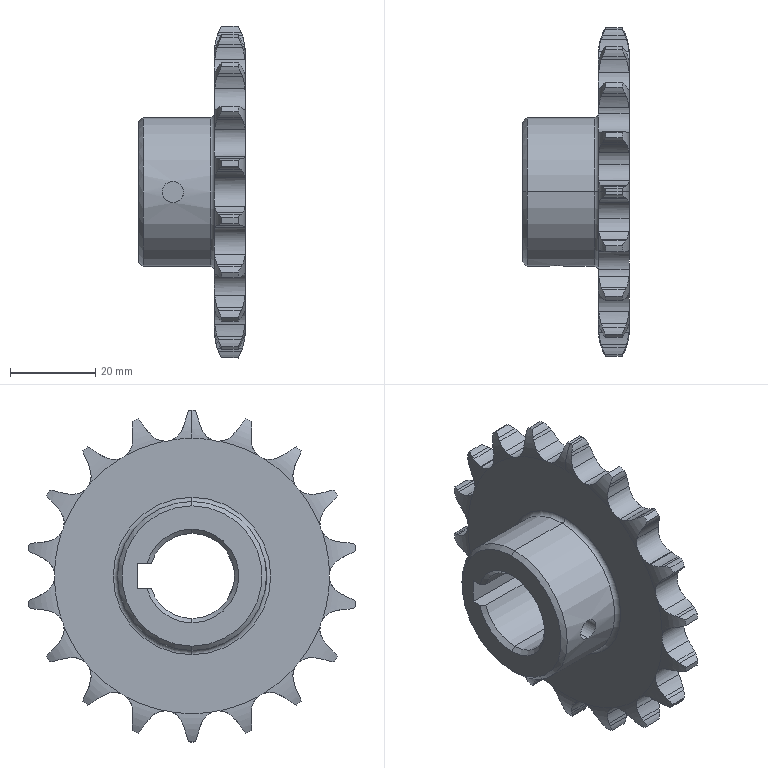Part | SolidWorks | features BaseBody 1 | 1 solid | 212 faces | box 25.007 x 77.055 x 78 mm | volume 35476 mm3 | cylinder 122 | plane 42 | torus 40 | cone 8 | commonest cylinder face diameters 12.41 x36 22.269 x36 8.653 x24 78 x19 20 x3 5 x2